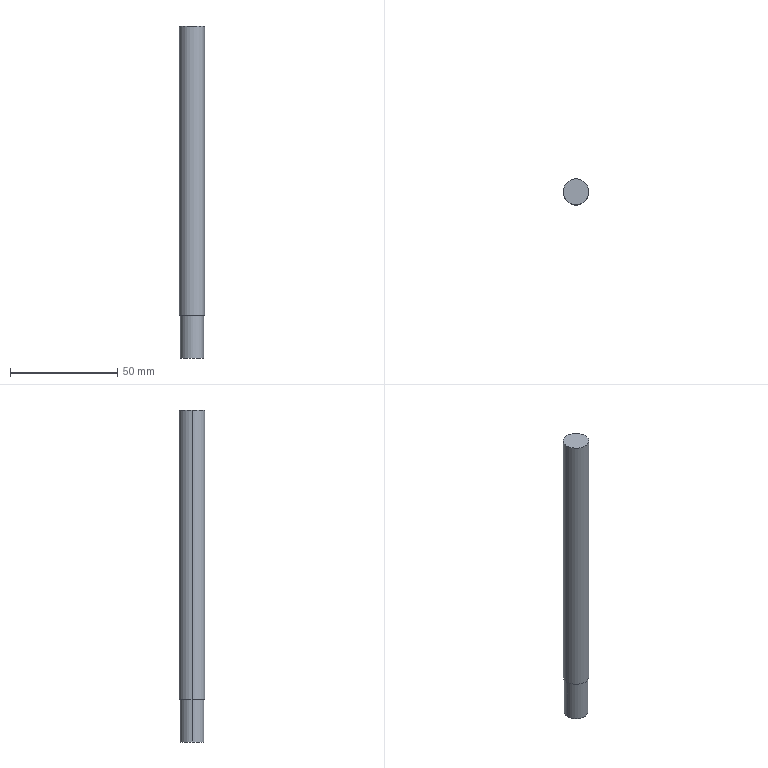Part | SolidWorks | features MirrorStock 1 | 1 solid | 7 faces | box 12 x 12 x 155 mm | volume 17169 mm3 | cylinder 4 | plane 3 | commonest cylinder face diameters 11 x2 12 x2
STEP:
#1=CARTESIAN_POINT('',(-5.5,0.,-57.5));
#2=VERTEX_POINT('',#1);
#3=CARTESIAN_POINT('',(5.5,0.,-57.5));
#4=VERTEX_POINT('',#3);
#5=CARTESIAN_POINT('',(0.,0.,-57.5));
#6=DIRECTION('',(0.,0.,1.));
#7=DIRECTION('',(1.,0.,0.));
#8=AXIS2_PLACEMENT_3D('',#5,#6,#7);
#9=CIRCLE('',#8,5.5);
#10=EDGE_CURVE('',#2,#4,#9,.T.);
#11=ORIENTED_EDGE('',*,*,#10,.F.);
#12=CARTESIAN_POINT('',(-5.5,0.,-77.5));
#13=VERTEX_POINT('',#12);
#14=CARTESIAN_POINT('',(-5.5,0.,-57.5));
#15=DIRECTION('',(0.,0.,-1.));
#16=VECTOR('',#15,1000.);
#17=LINE('',#14,#16);
#18=EDGE_CURVE('',#2,#13,#17,.T.);
#19=ORIENTED_EDGE('',*,*,#18,.T.);
#20=CARTESIAN_POINT('',(5.5,0.,-77.5));
#21=VERTEX_POINT('',#20);
#22=CARTESIAN_POINT('',(0.,0.,-77.5));
#23=DIRECTION('',(0.,0.,1.));
#24=DIRECTION('',(1.,0.,0.));
#25=AXIS2_PLACEMENT_3D('',#22,#23,#24);
#26=CIRCLE('',#25,5.5);
#27=EDGE_CURVE('',#13,#21,#26,.T.);
#28=ORIENTED_EDGE('',*,*,#27,.T.);
#29=CARTESIAN_POINT('',(5.5,0.,-57.5));
#30=DIRECTION('',(0.,0.,-1.));
#31=VECTOR('',#30,1000.);
#32=LINE('',#29,#31);
#33=EDGE_CURVE('',#4,#21,#32,.T.);
#34=ORIENTED_EDGE('',*,*,#33,.F.);
#35=EDGE_LOOP('',(#11,#19,#28,#34));
#36=FACE_OUTER_BOUND('',#35,.T.);
#37=CARTESIAN_POINT('',(0.,0.,-57.5));
#38=DIRECTION('',(0.,0.,-1.));
#39=DIRECTION('',(1.,0.,0.));
#40=AXIS2_PLACEMENT_3D('',#37,#38,#39);
#41=CYLINDRICAL_SURFACE('',#40,5.5);
#42=ADVANCED_FACE('',(#36),#41,.T.);
#43=CARTESIAN_POINT('',(-6.,0.,-57.5));
#44=VERTEX_POINT('',#43);
#45=CARTESIAN_POINT('',(6.,0.,-57.5));
#46=VERTEX_POINT('',#45);
#47=CARTESIAN_POINT('',(0.,0.,-57.5));
#48=DIRECTION('',(0.,0.,1.));
#49=DIRECTION('',(1.,0.,0.));
#50=AXIS2_PLACEMENT_3D('',#47,#48,#49);
#51=CIRCLE('',#50,6.);
#52=EDGE_CURVE('',#44,#46,#51,.T.);
#53=ORIENTED_EDGE('',*,*,#52,.T.);
#54=CARTESIAN_POINT('',(6.,0.,77.5));
#55=VERTEX_POINT('',#54);
#56=CARTESIAN_POINT('',(6.,0.,-77.5));
#57=DIRECTION('',(0.,0.,1.));
#58=VECTOR('',#57,1000.);
#59=LINE('',#56,#58);
#60=EDGE_CURVE('',#46,#55,#59,.T.);
#61=ORIENTED_EDGE('',*,*,#60,.T.);
#62=CARTESIAN_POINT('',(-6.,0.,77.5));
#63=VERTEX_POINT('',#62);
#64=CARTESIAN_POINT('',(0.,0.,77.5));
#65=DIRECTION('',(0.,0.,1.));
#66=DIRECTION('',(1.,0.,0.));
#67=AXIS2_PLACEMENT_3D('',#64,#65,#66);
#68=CIRCLE('',#67,6.);
#69=EDGE_CURVE('',#63,#55,#68,.T.);
#70=ORIENTED_EDGE('',*,*,#69,.F.);
#71=CARTESIAN_POINT('',(-6.,0.,-77.5));
#72=DIRECTION('',(0.,0.,1.));
#73=VECTOR('',#72,1000.);
#74=LINE('',#71,#73);
#75=EDGE_CURVE('',#44,#63,#74,.T.);
#76=ORIENTED_EDGE('',*,*,#75,.F.);
#77=EDGE_LOOP('',(#53,#61,#70,#76));
#78=FACE_OUTER_BOUND('',#77,.T.);
#79=CARTESIAN_POINT('',(0.,0.,-77.5));
#80=DIRECTION('',(0.,0.,1.));
#81=DIRECTION('',(-1.,0.,0.));
#82=AXIS2_PLACEMENT_3D('',#79,#80,#81);
#83=CYLINDRICAL_SURFACE('',#82,6.);
#84=ADVANCED_FACE('',(#78),#83,.T.);
#85=ORIENTED_EDGE('',*,*,#60,.F.);
#86=CARTESIAN_POINT('',(0.,0.,-57.5));
#87=DIRECTION('',(0.,0.,1.));
#88=DIRECTION('',(1.,0.,0.));
#89=AXIS2_PLACEMENT_3D('',#86,#87,#88);
#90=CIRCLE('',#89,6.);
#91=EDGE_CURVE('',#46,#44,#90,.T.);
#92=ORIENTED_EDGE('',*,*,#91,.T.);
#93=ORIENTED_EDGE('',*,*,#75,.T.);
#94=CARTESIAN_POINT('',(0.,0.,77.5));
#95=DIRECTION('',(0.,0.,1.));
#96=DIRECTION('',(1.,0.,0.));
#97=AXIS2_PLACEMENT_3D('',#94,#95,#96);
#98=CIRCLE('',#97,6.);
#99=EDGE_CURVE('',#55,#63,#98,.T.);
#100=ORIENTED_EDGE('',*,*,#99,.F.);
#101=EDGE_LOOP('',(#85,#92,#93,#100));
#102=FACE_OUTER_BOUND('',#101,.T.);
#103=CARTESIAN_POINT('',(0.,0.,-77.5));
#104=DIRECTION('',(0.,0.,1.));
#105=DIRECTION('',(-1.,0.,0.));
#106=AXIS2_PLACEMENT_3D('',#103,#104,#105);
#107=CYLINDRICAL_SURFACE('',#106,6.);
#108=ADVANCED_FACE('',(#102),#107,.T.);
#109=ORIENTED_EDGE('',*,*,#69,.T.);
#110=ORIENTED_EDGE('',*,*,#99,.T.);
#111=EDGE_LOOP('',(#109,#110));
#112=FACE_OUTER_BOUND('',#111,.T.);
#113=CARTESIAN_POINT('',(0.,0.,77.5));
#114=DIRECTION('',(0.,0.,-1.));
#115=DIRECTION('',(1.,0.,0.));
#116=AXIS2_PLACEMENT_3D('',#113,#114,#115);
#117=PLANE('',#116);
#118=ADVANCED_FACE('',(#112),#117,.F.);
#119=CARTESIAN_POINT('',(0.,0.,-57.5));
#120=DIRECTION('',(0.,0.,1.));
#121=DIRECTION('',(1.,0.,0.));
#122=AXIS2_PLACEMENT_3D('',#119,#120,#121);
#123=CIRCLE('',#122,5.5);
#124=EDGE_CURVE('',#4,#2,#123,.T.);
#125=ORIENTED_EDGE('',*,*,#124,.T.);
#126=ORIENTED_EDGE('',*,*,#10,.T.);
#127=EDGE_LOOP('',(#125,#126));
#128=FACE_BOUND('',#127,.T.);
#129=ORIENTED_EDGE('',*,*,#52,.F.);
#130=ORIENTED_EDGE('',*,*,#91,.F.);
#131=EDGE_LOOP('',(#129,#130));
#132=FACE_OUTER_BOUND('',#131,.T.);
#133=CARTESIAN_POINT('',(0.,0.,-57.5));
#134=DIRECTION('',(0.,0.,-1.));
#135=DIRECTION('',(1.,0.,0.));
#136=AXIS2_PLACEMENT_3D('',#133,#134,#135);
#137=PLANE('',#136);
#138=ADVANCED_FACE('',(#128,#132),#137,.T.);
#139=ORIENTED_EDGE('',*,*,#18,.F.);
#140=ORIENTED_EDGE('',*,*,#124,.F.);
#141=ORIENTED_EDGE('',*,*,#33,.T.);
#142=CARTESIAN_POINT('',(0.,0.,-77.5));
#143=DIRECTION('',(0.,0.,1.));
#144=DIRECTION('',(1.,0.,0.));
#145=AXIS2_PLACEMENT_3D('',#142,#143,#144);
#146=CIRCLE('',#145,5.5);
#147=EDGE_CURVE('',#21,#13,#146,.T.);
#148=ORIENTED_EDGE('',*,*,#147,.T.);
#149=EDGE_LOOP('',(#139,#140,#141,#148));
#150=FACE_OUTER_BOUND('',#149,.T.);
#151=CARTESIAN_POINT('',(0.,0.,-57.5));
#152=DIRECTION('',(0.,0.,-1.));
#153=DIRECTION('',(1.,0.,0.));
#154=AXIS2_PLACEMENT_3D('',#151,#152,#153);
#155=CYLINDRICAL_SURFACE('',#154,5.5);
#156=ADVANCED_FACE('',(#150),#155,.T.);
#157=ORIENTED_EDGE('',*,*,#147,.F.);
#158=ORIENTED_EDGE('',*,*,#27,.F.);
#159=EDGE_LOOP('',(#157,#158));
#160=FACE_OUTER_BOUND('',#159,.T.);
#161=CARTESIAN_POINT('',(0.,0.,-77.5));
#162=DIRECTION('',(0.,0.,-1.));
#163=DIRECTION('',(1.,0.,0.));
#164=AXIS2_PLACEMENT_3D('',#161,#162,#163);
#165=PLANE('',#164);
#166=ADVANCED_FACE('',(#160),#165,.T.);
#167=CLOSED_SHELL('',(#42,#84,#108,#118,#138,#156,#166));
#168=MANIFOLD_SOLID_BREP('',#167);
#169=CARTESIAN_POINT('',(0.,0.,0.));
#170=DIRECTION('',(0.,0.,1.));
#171=DIRECTION('',(1.,0.,0.));
#172=AXIS2_PLACEMENT_3D('',#169,#170,#171);
#173=(LENGTH_UNIT()NAMED_UNIT(*)SI_UNIT(.MILLI.,.METRE.));
#174=UNCERTAINTY_MEASURE_WITH_UNIT(LENGTH_MEASURE(0.00001),#173,'','');
#175=(NAMED_UNIT(*)PLANE_ANGLE_UNIT()SI_UNIT($,.RADIAN.));
#176=(NAMED_UNIT(*)SI_UNIT($,.STERADIAN.)SOLID_ANGLE_UNIT());
#177=(GEOMETRIC_REPRESENTATION_CONTEXT(3)GLOBAL_UNCERTAINTY_ASSIGNED_CONTEXT((#174))GLOBAL_UNIT_ASSIGNED_CONTEXT((#173,#175,#176))REPRESENTATION_CONTEXT('',''));
#178=ADVANCED_BREP_SHAPE_REPRESENTATION('',(#168,#172),#177);